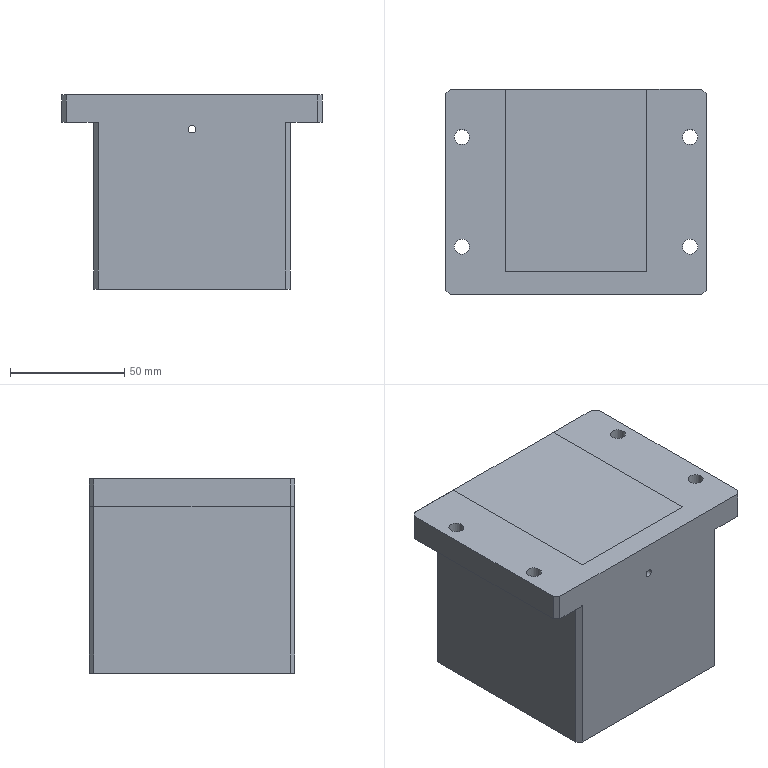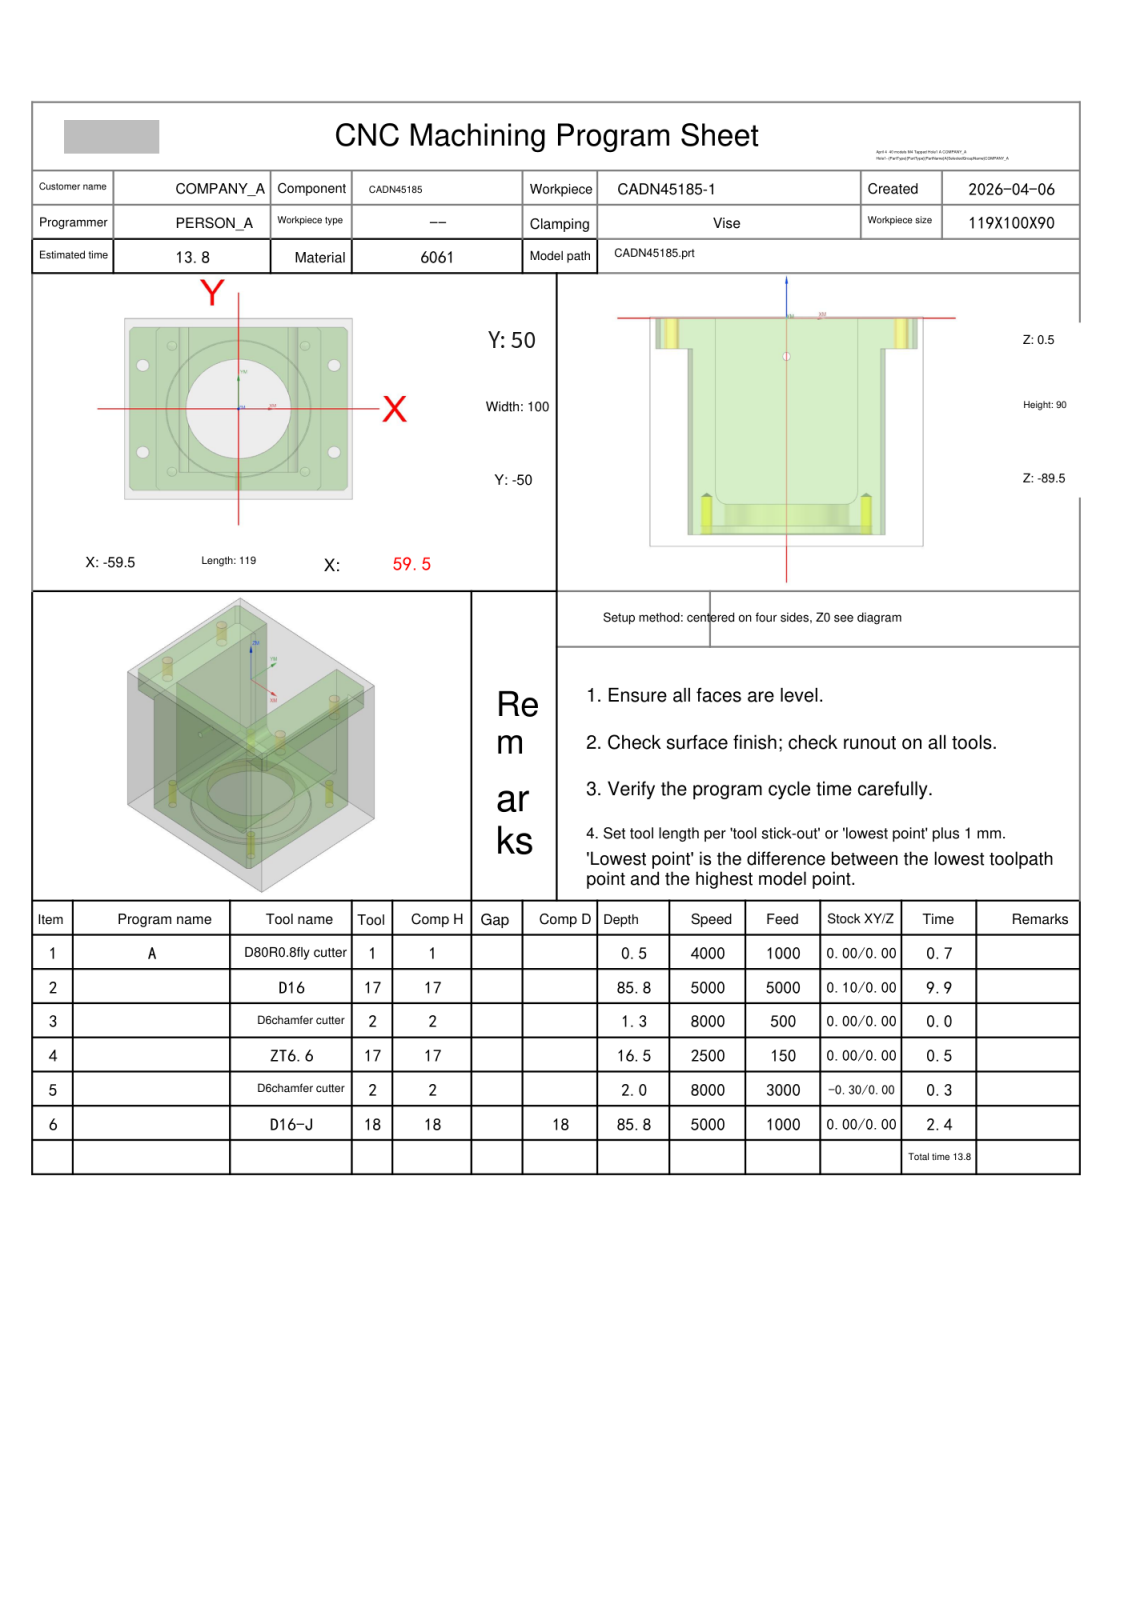NC program | NX | posted by the shop | part box 114 x 90 x 85 mm
Lines 35 to 791 of 2085:
N2 T17 M06
(D16  D=16. R=0. H=17 ce=0.10 di=0.00)
G00 G90 G54 X0.0 Y53.1 M03 S5000
G43 H17 Z20.
M08
Z.5
G01 X55. Z.404 F5000.
G02 X60.728 Y50.728 Z.393 I0.0 J-8.1
G01 X62.728 Y48.728 Z.388
G02 X65.1 Y43. Z.377 I-5.728 J-5.728
G01 Y-43. Z.226
G02 X62.728 Y-48.728 Z.215 I-8.1 J0.0
G01 X60.728 Y-50.728 Z.21
G02 X55. Y-53.1 Z.199 I-5.728 J5.728
G01 X-55. Z.007
G02 X-60.728 Y-50.728 Z-.005 I0.0 J8.1
G01 X-62.728 Y-48.728 Z-.009
G02 X-65.1 Y-43. Z-.021 I5.728 J5.728
G01 Y43. Z-.171
G02 X-62.728 Y48.728 Z-.182 I8.1 J0.0
G01 X-60.728 Y50.728 Z-.187
G02 X-55. Y53.1 Z-.198 I5.728 J-5.728
G01 X55. Z-.391
G02 X60.728 Y50.728 Z-.402 I0.0 J-8.1
G01 X62.728 Y48.728 Z-.407
G02 X65.1 Y43. Z-.418 I-5.728 J-5.728
G01 Y-43. Z-.568
G02 X62.728 Y-48.728 Z-.579 I-8.1 J0.0
G01 X60.728 Y-50.728 Z-.584
G02 X55. Y-53.1 Z-.595 I-5.728 J5.728
G01 X-55. Z-.788
G02 X-60.728 Y-50.728 Z-.799 I0.0 J8.1
G01 X-62.728 Y-48.728 Z-.804
G02 X-65.1 Y-43. Z-.815 I5.728 J5.728
G01 Y43. Z-.965
G02 X-62.728 Y48.728 Z-.977 I8.1 J0.0
G01 X-60.728 Y50.728 Z-.982
G02 X-55. Y53.1 Z-.993 I5.728 J-5.728
G01 X55. Z-1.185
G02 X60.728 Y50.728 Z-1.196 I0.0 J-8.1
G01 X62.728 Y48.728 Z-1.201
G02 X65.1 Y43. Z-1.212 I-5.728 J-5.728
G01 Y-43. Z-1.363
G02 X62.728 Y-48.728 Z-1.374 I-8.1 J0.0
G01 X60.728 Y-50.728 Z-1.379
G02 X55. Y-53.1 Z-1.39 I-5.728 J5.728
G01 X-55. Z-1.582
G02 X-60.728 Y-50.728 Z-1.593 I0.0 J8.1
G01 X-62.728 Y-48.728 Z-1.598
G02 X-65.1 Y-43. Z-1.61 I5.728 J5.728
G01 Y43. Z-1.76
G02 X-62.728 Y48.728 Z-1.771 I8.1 J0.0
G01 X-60.728 Y50.728 Z-1.776
G02 X-55. Y53.1 Z-1.787 I5.728 J-5.728
G01 X55. Z-1.98
G02 X60.728 Y50.728 Z-1.991 I0.0 J-8.1
G01 X62.728 Y48.728 Z-1.996
G02 X65.1 Y43. Z-2.007 I-5.728 J-5.728
G01 Y-43. Z-2.157
G02 X62.728 Y-48.728 Z-2.168 I-8.1 J0.0
G01 X60.728 Y-50.728 Z-2.173
G02 X55. Y-53.1 Z-2.184 I-5.728 J5.728
G01 X-55. Z-2.377
G02 X-60.728 Y-50.728 Z-2.388 I0.0 J8.1
G01 X-62.728 Y-48.728 Z-2.393
G02 X-65.1 Y-43. Z-2.404 I5.728 J5.728
G01 Y43. Z-2.554
G02 X-62.728 Y48.728 Z-2.566 I8.1 J0.0
G01 X-60.728 Y50.728 Z-2.57
G02 X-55. Y53.1 Z-2.582 I5.728 J-5.728
G01 X55. Z-2.774
G02 X60.728 Y50.728 Z-2.785 I0.0 J-8.1
G01 X62.728 Y48.728 Z-2.79
G02 X65.1 Y43. Z-2.801 I-5.728 J-5.728
G01 Y-43. Z-2.952
G02 X62.728 Y-48.728 Z-2.963 I-8.1 J0.0
G01 X60.728 Y-50.728 Z-2.968
G02 X55. Y-53.1 Z-2.979 I-5.728 J5.728
G01 X-55. Z-3.171
G02 X-60.728 Y-50.728 Z-3.182 I0.0 J8.1
G01 X-62.728 Y-48.728 Z-3.187
G02 X-65.1 Y-43. Z-3.198 I5.728 J5.728
G01 Y43. Z-3.349
G02 X-62.728 Y48.728 Z-3.36 I8.1 J0.0
G01 X-60.728 Y50.728 Z-3.365
G02 X-55. Y53.1 Z-3.376 I5.728 J-5.728
G01 X55. Z-3.568
G02 X60.728 Y50.728 Z-3.58 I0.0 J-8.1
G01 X62.728 Y48.728 Z-3.584
G02 X65.1 Y43. Z-3.596 I-5.728 J-5.728
G01 Y-43. Z-3.746
G02 X62.728 Y-48.728 Z-3.757 I-8.1 J0.0
G01 X60.728 Y-50.728 Z-3.762
G02 X55. Y-53.1 Z-3.773 I-5.728 J5.728
G01 X-55. Z-3.966
G02 X-60.728 Y-50.728 Z-3.977 I0.0 J8.1
G01 X-62.728 Y-48.728 Z-3.982
G02 X-65.1 Y-43. Z-3.993 I5.728 J5.728
G01 Y43. Z-4.143
G02 X-62.728 Y48.728 Z-4.154 I8.1 J0.0
G01 X-60.728 Y50.728 Z-4.159
G02 X-55. Y53.1 Z-4.17 I5.728 J-5.728
G01 X55. Z-4.363
G02 X60.728 Y50.728 Z-4.374 I0.0 J-8.1
G01 X62.728 Y48.728 Z-4.379
G02 X65.1 Y43. Z-4.39 I-5.728 J-5.728
G01 Y-43. Z-4.54
G02 X62.728 Y-48.728 Z-4.552 I-8.1 J0.0
G01 X60.728 Y-50.728 Z-4.557
G02 X55. Y-53.1 Z-4.568 I-5.728 J5.728
G01 X-55. Z-4.76
G02 X-60.728 Y-50.728 Z-4.771 I0.0 J8.1
G01 X-62.728 Y-48.728 Z-4.776
G02 X-65.1 Y-43. Z-4.787 I5.728 J5.728
G01 Y43. Z-4.938
G02 X-62.728 Y48.728 Z-4.949 I8.1 J0.0
G01 X-60.728 Y50.728 Z-4.954
G02 X-55. Y53.1 Z-4.965 I5.728 J-5.728
G01 X55. Z-5.157
G02 X60.728 Y50.728 Z-5.168 I0.0 J-8.1
G01 X62.728 Y48.728 Z-5.173
G02 X65.1 Y43. Z-5.185 I-5.728 J-5.728
G01 Y-43. Z-5.335
G02 X62.728 Y-48.728 Z-5.346 I-8.1 J0.0
G01 X60.728 Y-50.728 Z-5.351
G02 X55. Y-53.1 Z-5.362 I-5.728 J5.728
G01 X-55. Z-5.555
G02 X-60.728 Y-50.728 Z-5.566 I0.0 J8.1
G01 X-62.728 Y-48.728 Z-5.571
G02 X-65.1 Y-43. Z-5.582 I5.728 J5.728
G01 Y43. Z-5.732
G02 X-62.728 Y48.728 Z-5.743 I8.1 J0.0
G01 X-60.728 Y50.728 Z-5.748
G02 X-55. Y53.1 Z-5.759 I5.728 J-5.728
G01 X55. Z-5.952
G02 X60.728 Y50.728 Z-5.963 I0.0 J-8.1
G01 X62.728 Y48.728 Z-5.968
G02 X65.1 Y43. Z-5.979 I-5.728 J-5.728
G01 Y-43. Z-6.129
G02 X62.728 Y-48.728 Z-6.141 I-8.1 J0.0
G01 X60.728 Y-50.728 Z-6.145
G02 X55. Y-53.1 Z-6.157 I-5.728 J5.728
G01 X-55. Z-6.349
G02 X-60.728 Y-50.728 Z-6.36 I0.0 J8.1
G01 X-62.728 Y-48.728 Z-6.365
G02 X-65.1 Y-43. Z-6.376 I5.728 J5.728
G01 Y43. Z-6.527
G02 X-62.728 Y48.728 Z-6.538 I8.1 J0.0
G01 X-60.728 Y50.728 Z-6.543
G02 X-55. Y53.1 Z-6.554 I5.728 J-5.728
G01 X55. Z-6.746
G02 X60.728 Y50.728 Z-6.757 I0.0 J-8.1
G01 X62.728 Y48.728 Z-6.762
G02 X65.1 Y43. Z-6.773 I-5.728 J-5.728
G01 Y-43. Z-6.924
G02 X62.728 Y-48.728 Z-6.935 I-8.1 J0.0
G01 X60.728 Y-50.728 Z-6.94
G02 X55. Y-53.1 Z-6.951 I-5.728 J5.728
G01 X-55. Z-7.143
G02 X-60.728 Y-50.728 Z-7.155 I0.0 J8.1
G01 X-62.728 Y-48.728 Z-7.159
G02 X-65.1 Y-43. Z-7.171 I5.728 J5.728
G01 Y43. Z-7.321
G02 X-62.728 Y48.728 Z-7.332 I8.1 J0.0
G01 X-60.728 Y50.728 Z-7.337
G02 X-55. Y53.1 Z-7.348 I5.728 J-5.728
G01 X55. Z-7.541
G02 X60.728 Y50.728 Z-7.552 I0.0 J-8.1
G01 X62.728 Y48.728 Z-7.557
G02 X65.1 Y43. Z-7.568 I-5.728 J-5.728
G01 Y-43. Z-7.718
G02 X62.728 Y-48.728 Z-7.729 I-8.1 J0.0
G01 X60.728 Y-50.728 Z-7.734
G02 X55. Y-53.1 Z-7.745 I-5.728 J5.728
G01 X-55. Z-7.938
G02 X-60.728 Y-50.728 Z-7.949 I0.0 J8.1
G01 X-62.728 Y-48.728 Z-7.954
G02 X-65.1 Y-43. Z-7.965 I5.728 J5.728
G01 Y43. Z-8.115
G02 X-62.728 Y48.728 Z-8.127 I8.1 J0.0
G01 X-60.728 Y50.728 Z-8.132
G02 X-55. Y53.1 Z-8.143 I5.728 J-5.728
G01 X55. Z-8.335
G02 X60.728 Y50.728 Z-8.346 I0.0 J-8.1
G01 X62.728 Y48.728 Z-8.351
G02 X65.1 Y43. Z-8.362 I-5.728 J-5.728
G01 Y-43. Z-8.513
G02 X62.728 Y-48.728 Z-8.524 I-8.1 J0.0
G01 X60.728 Y-50.728 Z-8.529
G02 X55. Y-53.1 Z-8.54 I-5.728 J5.728
G01 X-55. Z-8.732
G02 X-60.728 Y-50.728 Z-8.743 I0.0 J8.1
G01 X-62.728 Y-48.728 Z-8.748
G02 X-65.1 Y-43. Z-8.76 I5.728 J5.728
G01 Y43. Z-8.91
G02 X-62.728 Y48.728 Z-8.921 I8.1 J0.0
G01 X-60.728 Y50.728 Z-8.926
G02 X-55. Y53.1 Z-8.937 I5.728 J-5.728
G01 X55. Z-9.13
G02 X60.728 Y50.728 Z-9.141 I0.0 J-8.1
G01 X62.728 Y48.728 Z-9.146
G02 X65.1 Y43. Z-9.157 I-5.728 J-5.728
G01 Y-43. Z-9.307
G02 X62.728 Y-48.728 Z-9.318 I-8.1 J0.0
G01 X60.728 Y-50.728 Z-9.323
G02 X55. Y-53.1 Z-9.334 I-5.728 J5.728
G01 X-55. Z-9.527
G02 X-60.728 Y-50.728 Z-9.538 I0.0 J8.1
G01 X-62.728 Y-48.728 Z-9.543
G02 X-65.1 Y-43. Z-9.554 I5.728 J5.728
G01 Y43. Z-9.704
G02 X-62.728 Y48.728 Z-9.716 I8.1 J0.0
G01 X-60.728 Y50.728 Z-9.72
G02 X-55. Y53.1 Z-9.732 I5.728 J-5.728
G01 X55. Z-9.924
G02 X60.728 Y50.728 Z-9.935 I0.0 J-8.1
G01 X62.728 Y48.728 Z-9.94
G02 X65.1 Y43. Z-9.951 I-5.728 J-5.728
G01 Y-43. Z-10.102
G02 X62.728 Y-48.728 Z-10.113 I-8.1 J0.0
G01 X60.728 Y-50.728 Z-10.118
G02 X55. Y-53.1 Z-10.129 I-5.728 J5.728
G01 X-55. Z-10.321
G02 X-60.728 Y-50.728 Z-10.332 I0.0 J8.1
G01 X-62.728 Y-48.728 Z-10.337
G02 X-65.1 Y-43. Z-10.348 I5.728 J5.728
G01 Y43. Z-10.499
G02 X-62.728 Y48.728 Z-10.51 I8.1 J0.0
G01 X-60.728 Y50.728 Z-10.515
G02 X-55. Y53.1 Z-10.526 I5.728 J-5.728
G01 X55. Z-10.718
G02 X60.728 Y50.728 Z-10.73 I0.0 J-8.1
G01 X62.728 Y48.728 Z-10.734
G02 X65.1 Y43. Z-10.746 I-5.728 J-5.728
G01 Y-43. Z-10.896
G02 X62.728 Y-48.728 Z-10.907 I-8.1 J0.0
G01 X60.728 Y-50.728 Z-10.912
G02 X55. Y-53.1 Z-10.923 I-5.728 J5.728
G01 X-55. Z-11.116
G02 X-60.728 Y-50.728 Z-11.127 I0.0 J8.1
G01 X-62.728 Y-48.728 Z-11.132
G02 X-65.1 Y-43. Z-11.143 I5.728 J5.728
G01 Y43. Z-11.293
G02 X-62.728 Y48.728 Z-11.304 I8.1 J0.0
G01 X-60.728 Y50.728 Z-11.309
G02 X-55. Y53.1 Z-11.32 I5.728 J-5.728
G01 X55. Z-11.513
G02 X60.728 Y50.728 Z-11.524 I0.0 J-8.1
G01 X62.728 Y48.728 Z-11.529
G02 X65.1 Y43. Z-11.54 I-5.728 J-5.728
G01 Y-43. Z-11.69
G02 X62.728 Y-48.728 Z-11.702 I-8.1 J0.0
G01 X60.728 Y-50.728 Z-11.707
G02 X55. Y-53.1 Z-11.718 I-5.728 J5.728
G01 X-55. Z-11.91
G02 X-60.728 Y-50.728 Z-11.921 I0.0 J8.1
G01 X-62.728 Y-48.728 Z-11.926
G02 X-65.1 Y-43. Z-11.937 I5.728 J5.728
G01 Y43. Z-12.088
G02 X-62.728 Y48.728 Z-12.099 I8.1 J0.0
G01 X-60.728 Y50.728 Z-12.104
G02 X-55. Y53.1 Z-12.115 I5.728 J-5.728
G01 X55. Z-12.307
G02 X60.728 Y50.728 Z-12.318 I0.0 J-8.1
G01 X62.728 Y48.728 Z-12.323
G02 X65.1 Y43. Z-12.335 I-5.728 J-5.728
G01 Y-43. Z-12.485
G02 X62.728 Y-48.728 Z-12.496 I-8.1 J0.0
G01 X60.728 Y-50.728 Z-12.501
G02 X55. Y-53.1 Z-12.512 I-5.728 J5.728
G01 X-55. Z-12.705
G02 X-60.728 Y-50.728 Z-12.716 I0.0 J8.1
G01 X-62.728 Y-48.728 Z-12.721
G02 X-65.1 Y-43. Z-12.732 I5.728 J5.728
G01 Y43. Z-12.882
G02 X-62.728 Y48.728 Z-12.893 I8.1 J0.0
G01 X-60.728 Y50.728 Z-12.898
G02 X-55. Y53.1 Z-12.909 I5.728 J-5.728
G01 X55. Z-13.102
G02 X60.728 Y50.728 Z-13.113 I0.0 J-8.1
G01 X62.728 Y48.728 Z-13.118
G02 X65.1 Y43. Z-13.129 I-5.728 J-5.728
G01 Y-43. Z-13.279
G02 X62.728 Y-48.728 Z-13.291 I-8.1 J0.0
G01 X60.728 Y-50.728 Z-13.295
G02 X55. Y-53.1 Z-13.307 I-5.728 J5.728
G01 X-55. Z-13.499
G02 X-60.728 Y-50.728 Z-13.51 I0.0 J8.1
G01 X-62.728 Y-48.728 Z-13.515
G02 X-65.1 Y-43. Z-13.526 I5.728 J5.728
G01 Y43. Z-13.677
G02 X-62.728 Y48.728 Z-13.688 I8.1 J0.0
G01 X-60.728 Y50.728 Z-13.693
G02 X-55. Y53.1 Z-13.704 I5.728 J-5.728
G01 X55. Z-13.896
G02 X60.728 Y50.728 Z-13.907 I0.0 J-8.1
G01 X62.728 Y48.728 Z-13.912
G02 X65.1 Y43. Z-13.923 I-5.728 J-5.728
G01 Y-43. Z-14.074
G02 X62.728 Y-48.728 Z-14.085 I-8.1 J0.0
G01 X60.728 Y-50.728 Z-14.09
G02 X55. Y-53.1 Z-14.101 I-5.728 J5.728
G01 X-55. Z-14.293
G02 X-60.728 Y-50.728 Z-14.305 I0.0 J8.1
G01 X-62.728 Y-48.728 Z-14.309
G02 X-65.1 Y-43. Z-14.321 I5.728 J5.728
G01 Y43. Z-14.471
G02 X-62.728 Y48.728 Z-14.482 I8.1 J0.0
G01 X-60.728 Y50.728 Z-14.487
G02 X-55. Y53.1 Z-14.498 I5.728 J-5.728
G01 X55. Z-14.691
G02 X60.728 Y50.728 Z-14.702 I0.0 J-8.1
G01 X62.728 Y48.728 Z-14.707
G02 X65.1 Y43. Z-14.718 I-5.728 J-5.728
G01 Y-43. Z-14.868
G02 X62.728 Y-48.728 Z-14.879 I-8.1 J0.0
G01 X60.728 Y-50.728 Z-14.884
G02 X55. Y-53.1 Z-14.895 I-5.728 J5.728
G01 X-55. Z-15.088
G02 X-60.728 Y-50.728 Z-15.099 I0.0 J8.1
G01 X-62.728 Y-48.728 Z-15.104
G02 X-65.1 Y-43. Z-15.115 I5.728 J5.728
G01 Y43. Z-15.265
G02 X-62.728 Y48.728 Z-15.277 I8.1 J0.0
G01 X-60.728 Y50.728 Z-15.282
G02 X-55. Y53.1 Z-15.293 I5.728 J-5.728
G01 X55. Z-15.485
G02 X60.728 Y50.728 Z-15.496 I0.0 J-8.1
G01 X62.728 Y48.728 Z-15.501
G02 X65.1 Y43. Z-15.512 I-5.728 J-5.728
G01 Y-43. Z-15.663
G02 X62.728 Y-48.728 Z-15.674 I-8.1 J0.0
G01 X60.728 Y-50.728 Z-15.679
G02 X55. Y-53.1 Z-15.69 I-5.728 J5.728
G01 X-55. Z-15.882
G02 X-60.728 Y-50.728 Z-15.893 I0.0 J8.1
G01 X-62.728 Y-48.728 Z-15.898
G02 X-65.1 Y-43. Z-15.91 I5.728 J5.728
G01 Y43. Z-16.06
G02 X-62.728 Y48.728 Z-16.071 I8.1 J0.0
G01 X-60.728 Y50.728 Z-16.076
G02 X-55. Y53.1 Z-16.087 I5.728 J-5.728
G01 X55. Z-16.28
G02 X60.728 Y50.728 Z-16.291 I0.0 J-8.1
G01 X62.728 Y48.728 Z-16.296
G02 X65.1 Y43. Z-16.307 I-5.728 J-5.728
G01 Y-43. Z-16.457
G02 X62.728 Y-48.728 Z-16.468 I-8.1 J0.0
G01 X60.728 Y-50.728 Z-16.473
G02 X55. Y-53.1 Z-16.484 I-5.728 J5.728
G01 X-55. Z-16.677
G02 X-60.728 Y-50.728 Z-16.688 I0.0 J8.1
G01 X-62.728 Y-48.728 Z-16.693
G02 X-65.1 Y-43. Z-16.704 I5.728 J5.728
G01 Y43. Z-16.854
G02 X-62.728 Y48.728 Z-16.866 I8.1 J0.0
G01 X-60.728 Y50.728 Z-16.87
G02 X-55. Y53.1 Z-16.882 I5.728 J-5.728
G01 X55. Z-17.074
G02 X60.728 Y50.728 Z-17.085 I0.0 J-8.1
G01 X62.728 Y48.728 Z-17.09
G02 X65.1 Y43. Z-17.101 I-5.728 J-5.728
G01 Y-43. Z-17.252
G02 X62.728 Y-48.728 Z-17.263 I-8.1 J0.0
G01 X60.728 Y-50.728 Z-17.268
G02 X55. Y-53.1 Z-17.279 I-5.728 J5.728
G01 X-55. Z-17.471
G02 X-60.728 Y-50.728 Z-17.482 I0.0 J8.1
G01 X-62.728 Y-48.728 Z-17.487
G02 X-65.1 Y-43. Z-17.498 I5.728 J5.728
G01 Y43. Z-17.649
G02 X-62.728 Y48.728 Z-17.66 I8.1 J0.0
G01 X-60.728 Y50.728 Z-17.665
G02 X-55. Y53.1 Z-17.676 I5.728 J-5.728
G01 X55. Z-17.868
G02 X60.728 Y50.728 Z-17.88 I0.0 J-8.1
G01 X62.728 Y48.728 Z-17.884
G02 X65.1 Y43. Z-17.896 I-5.728 J-5.728
G01 Y-43. Z-18.046
G02 X62.728 Y-48.728 Z-18.057 I-8.1 J0.0
G01 X60.728 Y-50.728 Z-18.062
G02 X55. Y-53.1 Z-18.073 I-5.728 J5.728
G01 X-55. Z-18.266
G02 X-60.728 Y-50.728 Z-18.277 I0.0 J8.1
G01 X-62.728 Y-48.728 Z-18.282
G02 X-65.1 Y-43. Z-18.293 I5.728 J5.728
G01 Y43. Z-18.443
G02 X-62.728 Y48.728 Z-18.454 I8.1 J0.0
G01 X-60.728 Y50.728 Z-18.459
G02 X-55. Y53.1 Z-18.47 I5.728 J-5.728
G01 X55. Z-18.663
G02 X60.728 Y50.728 Z-18.674 I0.0 J-8.1
G01 X62.728 Y48.728 Z-18.679
G02 X65.1 Y43. Z-18.69 I-5.728 J-5.728
G01 Y-43. Z-18.84
G02 X62.728 Y-48.728 Z-18.852 I-8.1 J0.0
G01 X60.728 Y-50.728 Z-18.857
G02 X55. Y-53.1 Z-18.868 I-5.728 J5.728
G01 X-55. Z-19.06
G02 X-60.728 Y-50.728 Z-19.071 I0.0 J8.1
G01 X-62.728 Y-48.728 Z-19.076
G02 X-65.1 Y-43. Z-19.087 I5.728 J5.728
G01 Y43. Z-19.238
G02 X-62.728 Y48.728 Z-19.249 I8.1 J0.0
G01 X-60.728 Y50.728 Z-19.254
G02 X-55. Y53.1 Z-19.265 I5.728 J-5.728
G01 X55. Z-19.457
G02 X60.728 Y50.728 Z-19.468 I0.0 J-8.1
G01 X62.728 Y48.728 Z-19.473
G02 X65.1 Y43. Z-19.485 I-5.728 J-5.728
G01 Y-43. Z-19.635
G02 X62.728 Y-48.728 Z-19.646 I-8.1 J0.0
G01 X60.728 Y-50.728 Z-19.651
G02 X55. Y-53.1 Z-19.662 I-5.728 J5.728
G01 X-55. Z-19.855
G02 X-60.728 Y-50.728 Z-19.866 I0.0 J8.1
G01 X-62.728 Y-48.728 Z-19.871
G02 X-65.1 Y-43. Z-19.882 I5.728 J5.728
G01 Y43. Z-20.032
G02 X-62.728 Y48.728 Z-20.043 I8.1 J0.0
G01 X-60.728 Y50.728 Z-20.048
G02 X-55. Y53.1 Z-20.059 I5.728 J-5.728
G01 X55. Z-20.252
G02 X60.728 Y50.728 Z-20.263 I0.0 J-8.1
G01 X62.728 Y48.728 Z-20.268
G02 X65.1 Y43. Z-20.279 I-5.728 J-5.728
G01 Y-43. Z-20.429
G02 X62.728 Y-48.728 Z-20.441 I-8.1 J0.0
G01 X60.728 Y-50.728 Z-20.445
G02 X55. Y-53.1 Z-20.457 I-5.728 J5.728
G01 X-55. Z-20.649
G02 X-60.728 Y-50.728 Z-20.66 I0.0 J8.1
G01 X-62.728 Y-48.728 Z-20.665
G02 X-65.1 Y-43. Z-20.676 I5.728 J5.728
G01 Y43. Z-20.827
G02 X-62.728 Y48.728 Z-20.838 I8.1 J0.0
G01 X-60.728 Y50.728 Z-20.843
G02 X-55. Y53.1 Z-20.854 I5.728 J-5.728
G01 X55. Z-21.046
G02 X60.728 Y50.728 Z-21.057 I0.0 J-8.1
G01 X62.728 Y48.728 Z-21.062
G02 X65.1 Y43. Z-21.073 I-5.728 J-5.728
G01 Y-43. Z-21.224
G02 X62.728 Y-48.728 Z-21.235 I-8.1 J0.0
G01 X60.728 Y-50.728 Z-21.24
G02 X55. Y-53.1 Z-21.251 I-5.728 J5.728
G01 X-55. Z-21.443
G02 X-60.728 Y-50.728 Z-21.455 I0.0 J8.1
G01 X-62.728 Y-48.728 Z-21.459
G02 X-65.1 Y-43. Z-21.471 I5.728 J5.728
G01 Y43. Z-21.621
G02 X-62.728 Y48.728 Z-21.632 I8.1 J0.0
G01 X-60.728 Y50.728 Z-21.637
G02 X-55. Y53.1 Z-21.648 I5.728 J-5.728
G01 X55. Z-21.841
G02 X60.728 Y50.728 Z-21.852 I0.0 J-8.1
G01 X62.728 Y48.728 Z-21.857
G02 X65.1 Y43. Z-21.868 I-5.728 J-5.728
G01 Y-43. Z-22.018
G02 X62.728 Y-48.728 Z-22.029 I-8.1 J0.0
G01 X60.728 Y-50.728 Z-22.034
G02 X55. Y-53.1 Z-22.045 I-5.728 J5.728
G01 X-55. Z-22.238
G02 X-60.728 Y-50.728 Z-22.249 I0.0 J8.1
G01 X-62.728 Y-48.728 Z-22.254
G02 X-65.1 Y-43. Z-22.265 I5.728 J5.728
G01 Y43. Z-22.415
G02 X-62.728 Y48.728 Z-22.427 I8.1 J0.0
G01 X-60.728 Y50.728 Z-22.432
G02 X-55. Y53.1 Z-22.443 I5.728 J-5.728
G01 X55. Z-22.635
G02 X60.728 Y50.728 Z-22.646 I0.0 J-8.1
G01 X62.728 Y48.728 Z-22.651
G02 X65.1 Y43. Z-22.662 I-5.728 J-5.728
G01 Y-43. Z-22.813
G02 X62.728 Y-48.728 Z-22.824 I-8.1 J0.0
G01 X60.728 Y-50.728 Z-22.829
G02 X55. Y-53.1 Z-22.84 I-5.728 J5.728
G01 X-55. Z-23.032
G02 X-60.728 Y-50.728 Z-23.043 I0.0 J8.1
G01 X-62.728 Y-48.728 Z-23.048
G02 X-65.1 Y-43. Z-23.06 I5.728 J5.728
G01 Y43. Z-23.21
G02 X-62.728 Y48.728 Z-23.221 I8.1 J0.0
G01 X-60.728 Y50.728 Z-23.226
G02 X-55. Y53.1 Z-23.237 I5.728 J-5.728
G01 X55. Z-23.43
G02 X60.728 Y50.728 Z-23.441 I0.0 J-8.1
G01 X62.728 Y48.728 Z-23.446
G02 X65.1 Y43. Z-23.457 I-5.728 J-5.728
G01 Y-43. Z-23.607
G02 X62.728 Y-48.728 Z-23.618 I-8.1 J0.0
G01 X60.728 Y-50.728 Z-23.623
G02 X55. Y-53.1 Z-23.634 I-5.728 J5.728
G01 X-55. Z-23.827
G02 X-60.728 Y-50.728 Z-23.838 I0.0 J8.1
G01 X-62.728 Y-48.728 Z-23.843
G02 X-65.1 Y-43. Z-23.854 I5.728 J5.728
G01 Y43. Z-24.004
G02 X-62.728 Y48.728 Z-24.016 I8.1 J0.0
G01 X-60.728 Y50.728 Z-24.02
G02 X-55. Y53.1 Z-24.032 I5.728 J-5.728
G01 X55. Z-24.224
G02 X60.728 Y50.728 Z-24.235 I0.0 J-8.1
G01 X62.728 Y48.728 Z-24.24
G02 X65.1 Y43. Z-24.251 I-5.728 J-5.728
G01 Y-43. Z-24.402
G02 X62.728 Y-48.728 Z-24.413 I-8.1 J0.0
G01 X60.728 Y-50.728 Z-24.418
G02 X55. Y-53.1 Z-24.429 I-5.728 J5.728
G01 X-55. Z-24.621
G02 X-60.728 Y-50.728 Z-24.632 I0.0 J8.1
G01 X-62.728 Y-48.728 Z-24.637
G02 X-65.1 Y-43. Z-24.648 I5.728 J5.728
G01 Y43. Z-24.799
G02 X-62.728 Y48.728 Z-24.81 I8.1 J0.0
G01 X-60.728 Y50.728 Z-24.815
G02 X-55. Y53.1 Z-24.826 I5.728 J-5.728
G01 X55. Z-25.018
G02 X60.728 Y50.728 Z-25.03 I0.0 J-8.1
G01 X62.728 Y48.728 Z-25.034
G02 X65.1 Y43. Z-25.046 I-5.728 J-5.728
G01 Y-43. Z-25.196
G02 X62.728 Y-48.728 Z-25.207 I-8.1 J0.0
G01 X60.728 Y-50.728 Z-25.212
G02 X55. Y-53.1 Z-25.223 I-5.728 J5.728
G01 X-55. Z-25.416
G02 X-60.728 Y-50.728 Z-25.427 I0.0 J8.1
G01 X-62.728 Y-48.728 Z-25.432
G02 X-65.1 Y-43. Z-25.443 I5.728 J5.728
G01 Y43. Z-25.593
G02 X-62.728 Y48.728 Z-25.604 I8.1 J0.0
G01 X-60.728 Y50.728 Z-25.609
G02 X-55. Y53.1 Z-25.62 I5.728 J-5.728
G01 X55. Z-25.813
G02 X60.728 Y50.728 Z-25.824 I0.0 J-8.1
G01 X62.728 Y48.728 Z-25.829
G02 X65.1 Y43. Z-25.84 I-5.728 J-5.728
G01 Y-43. Z-25.99
G02 X62.728 Y-48.728 Z-26.002 I-8.1 J0.0
G01 X60.728 Y-50.728 Z-26.007
G02 X55. Y-53.1 Z-26.018 I-5.728 J5.728
G01 X-55. Z-26.21
G02 X-60.728 Y-50.728 Z-26.221 I0.0 J8.1
G01 X-62.728 Y-48.728 Z-26.226
G02 X-65.1 Y-43. Z-26.237 I5.728 J5.728
G01 Y43. Z-26.388
G02 X-62.728 Y48.728 Z-26.399 I8.1 J0.0
G01 X-60.728 Y50.728 Z-26.404
G02 X-55. Y53.1 Z-26.415 I5.728 J-5.728
G01 X55. Z-26.607
G02 X60.728 Y50.728 Z-26.618 I0.0 J-8.1
G01 X62.728 Y48.728 Z-26.623
G02 X65.1 Y43. Z-26.635 I-5.728 J-5.728
G01 Y-43. Z-26.785
G02 X62.728 Y-48.728 Z-26.796 I-8.1 J0.0
G01 X60.728 Y-50.728 Z-26.801
G02 X55. Y-53.1 Z-26.812 I-5.728 J5.728
G01 X-55. Z-27.005
G02 X-60.728 Y-50.728 Z-27.016 I0.0 J8.1
G01 X-62.728 Y-48.728 Z-27.021
G02 X-65.1 Y-43. Z-27.032 I5.728 J5.728
G01 Y43. Z-27.182
G02 X-62.728 Y48.728 Z-27.193 I8.1 J0.0
G01 X-60.728 Y50.728 Z-27.198
G02 X-55. Y53.1 Z-27.209 I5.728 J-5.728
G01 X55. Z-27.402
G02 X60.728 Y50.728 Z-27.413 I0.0 J-8.1
G01 X62.728 Y48.728 Z-27.418
G02 X65.1 Y43. Z-27.429 I-5.728 J-5.728
G01 Y-43. Z-27.579
G02 X62.728 Y-48.728 Z-27.591 I-8.1 J0.0
G01 X60.728 Y-50.728 Z-27.595
G02 X55. Y-53.1 Z-27.607 I-5.728 J5.728
G01 X-55. Z-27.799
G02 X-60.728 Y-50.728 Z-27.81 I0.0 J8.1
G01 X-62.728 Y-48.728 Z-27.815
G02 X-65.1 Y-43. Z-27.826 I5.728 J5.728
G01 Y43. Z-27.977
G02 X-62.728 Y48.728 Z-27.988 I8.1 J0.0
G01 X-60.728 Y50.728 Z-27.993
G02 X-55. Y53.1 Z-28.004 I5.728 J-5.728
G01 X55. Z-28.196
G02 X60.728 Y50.728 Z-28.207 I0.0 J-8.1
G01 X62.728 Y48.728 Z-28.212
G02 X65.1 Y43. Z-28.223 I-5.728 J-5.728
G01 Y-43. Z-28.374
G02 X62.728 Y-48.728 Z-28.385 I-8.1 J0.0
G01 X60.728 Y-50.728 Z-28.39
G02 X55. Y-53.1 Z-28.401 I-5.728 J5.728
G01 X-55. Z-28.593
G02 X-60.728 Y-50.728 Z-28.605 I0.0 J8.1
G01 X-62.728 Y-48.728 Z-28.609
G02 X-65.1 Y-43. Z-28.621 I5.728 J5.728
G01 Y43. Z-28.771
G02 X-62.728 Y48.728 Z-28.782 I8.1 J0.0
G01 X-60.728 Y50.728 Z-28.787
G02 X-55. Y53.1 Z-28.798 I5.728 J-5.728
G01 X55. Z-28.991
G02 X60.728 Y50.728 Z-29.002 I0.0 J-8.1
G01 X62.728 Y48.728 Z-29.007
G02 X65.1 Y43. Z-29.018 I-5.728 J-5.728
G01 Y-43. Z-29.168
G02 X62.728 Y-48.728 Z-29.179 I-8.1 J0.0
G01 X60.728 Y-50.728 Z-29.184
G02 X55. Y-53.1 Z-29.195 I-5.728 J5.728
G01 X-55. Z-29.388
G02 X-60.728 Y-50.728 Z-29.399 I0.0 J8.1
G01 X-62.728 Y-48.728 Z-29.404
G02 X-65.1 Y-43. Z-29.415 I5.728 J5.728
G01 Y43. Z-29.565
G02 X-62.728 Y48.728 Z-29.577 I8.1 J0.0
G01 X-60.728 Y50.728 Z-29.582
G02 X-55. Y53.1 Z-29.593 I5.728 J-5.728
G01 X55. Z-29.785
G02 X60.728 Y50.728 Z-29.796 I0.0 J-8.1
G01 X62.728 Y48.728 Z-29.801
G02 X65.1 Y43. Z-29.812 I-5.728 J-5.728
G01 Y-43. Z-29.963
G02 X62.728 Y-48.728 Z-29.974 I-8.1 J0.0
G01 X60.728 Y-50.728 Z-29.979
G02 X55. Y-53.1 Z-29.99 I-5.728 J5.728
G01 X-55. Z-30.182
G02 X-60.728 Y-50.728 Z-30.193 I0.0 J8.1
G01 X-62.728 Y-48.728 Z-30.198
G02 X-65.1 Y-43. Z-30.21 I5.728 J5.728
G01 Y43. Z-30.36
G02 X-62.728 Y48.728 Z-30.371 I8.1 J0.0
G01 X-60.728 Y50.728 Z-30.376
G02 X-55. Y53.1 Z-30.387 I5.728 J-5.728
G01 X55. Z-30.58
G02 X60.728 Y50.728 Z-30.591 I0.0 J-8.1
G01 X62.728 Y48.728 Z-30.596
G02 X65.1 Y43. Z-30.607 I-5.728 J-5.728
G01 Y-43. Z-30.757
G02 X62.728 Y-48.728 Z-30.768 I-8.1 J0.0
G01 X60.728 Y-50.728 Z-30.773
G02 X55. Y-53.1 Z-30.784 I-5.728 J5.728
G01 X-55. Z-30.977
G02 X-60.728 Y-50.728 Z-30.988 I0.0 J8.1
G01 X-62.728 Y-48.728 Z-30.993
G02 X-65.1 Y-43. Z-31.004 I5.728 J5.728
G01 Y43. Z-31.154
G02 X-62.728 Y48.728 Z-31.166 I8.1 J0.0
G01 X-60.728 Y50.728 Z-31.17
G02 X-55. Y53.1 Z-31.182 I5.728 J-5.728
G01 X55. Z-31.374
G02 X60.728 Y50.728 Z-31.385 I0.0 J-8.1
G01 X62.728 Y48.728 Z-31.39
G02 X65.1 Y43. Z-31.401 I-5.728 J-5.728
G01 Y-43. Z-31.552
G02 X62.728 Y-48.728 Z-31.563 I-8.1 J0.0
G01 X60.728 Y-50.728 Z-31.568
G02 X55. Y-53.1 Z-31.579 I-5.728 J5.728
G01 X-55. Z-31.771
G02 X-60.728 Y-50.728 Z-31.782 I0.0 J8.1
G01 X-62.728 Y-48.728 Z-31.787
G02 X-65.1 Y-43. Z-31.798 I5.728 J5.728
G01 Y43. Z-31.949
G02 X-62.728 Y48.728 Z-31.96 I8.1 J0.0
G01 X-60.728 Y50.728 Z-31.965
G02 X-55. Y53.1 Z-31.976 I5.728 J-5.728
G01 X55. Z-32.168
G02 X60.728 Y50.728 Z-32.18 I0.0 J-8.1
G01 X62.728 Y48.728 Z-32.184
G02 X65.1 Y43. Z-32.196 I-5.728 J-5.728
G01 Y-43. Z-32.346
G02 X62.728 Y-48.728 Z-32.357 I-8.1 J0.0
G01 X60.728 Y-50.728 Z-32.362
G02 X55. Y-53.1 Z-32.373 I-5.728 J5.728
G01 X-55. Z-32.566
G02 X-60.728 Y-50.728 Z-32.577 I0.0 J8.1
G01 X-62.728 Y-48.728 Z-32.582
G02 X-65.1 Y-43. Z-32.593 I5.728 J5.728
G01 Y43. Z-32.743
G02 X-62.728 Y48.728 Z-32.754 I8.1 J0.0
G01 X-60.728 Y50.728 Z-32.759
G02 X-55. Y53.1 Z-32.77 I5.728 J-5.728
G01 X55. Z-32.963
G02 X60.728 Y50.728 Z-32.974 I0.0 J-8.1
G01 X62.728 Y48.728 Z-32.979
G02 X65.1 Y43. Z-32.99 I-5.728 J-5.728
G01 Y-43. Z-33.14
G02 X62.728 Y-48.728 Z-33.152 I-8.1 J0.0
G01 X60.728 Y-50.728 Z-33.157
G02 X55. Y-53.1 Z-33.168 I-5.728 J5.728
G01 X-55. Z-33.36
G02 X-60.728 Y-50.728 Z-33.371 I0.0 J8.1
G01 X-62.728 Y-48.728 Z-33.376
G02 X-65.1 Y-43. Z-33.387 I5.728 J5.728
G01 Y43. Z-33.538
G02 X-62.728 Y48.728 Z-33.549 I8.1 J0.0
G01 X-60.728 Y50.728 Z-33.554
G02 X-55. Y53.1 Z-33.565 I5.728 J-5.728
G01 X55. Z-33.757
G02 X60.728 Y50.728 Z-33.768 I0.0 J-8.1
G01 X62.728 Y48.728 Z-33.773
G02 X65.1 Y43. Z-33.785 I-5.728 J-5.728
G01 Y-43. Z-33.935
G02 X62.728 Y-48.728 Z-33.946 I-8.1 J0.0
G01 X60.728 Y-50.728 Z-33.951
G02 X55. Y-53.1 Z-33.962 I-5.728 J5.728
G01 X-55. Z-34.155
G02 X-60.728 Y-50.728 Z-34.166 I0.0 J8.1
G01 X-62.728 Y-48.728 Z-34.171
G02 X-65.1 Y-43. Z-34.182 I5.728 J5.728
G01 Y43. Z-34.332
G02 X-62.728 Y48.728 Z-34.343 I8.1 J0.0
G01 X-60.728 Y50.728 Z-34.348
G02 X-55. Y53.1 Z-34.359 I5.728 J-5.728
G01 X55. Z-34.552
G02 X60.728 Y50.728 Z-34.563 I0.0 J-8.1
G01 X62.728 Y48.728 Z-34.568
G02 X65.1 Y43. Z-34.579 I-5.728 J-5.728
G01 Y-43. Z-34.729
G02 X62.728 Y-48.728 Z-34.741 I-8.1 J0.0
G01 X60.728 Y-50.728 Z-34.745
G02 X55. Y-53.1 Z-34.757 I-5.728 J5.728
G01 X-55. Z-34.949
G02 X-60.728 Y-50.728 Z-34.96 I0.0 J8.1
G01 X-62.728 Y-48.728 Z-34.965
G02 X-65.1 Y-43. Z-34.976 I5.728 J5.728
G01 Y43. Z-35.127
G02 X-62.728 Y48.728 Z-35.138 I8.1 J0.0
G01 X-60.728 Y50.728 Z-35.143
G02 X-55. Y53.1 Z-35.154 I5.728 J-5.728
G01 X55. Z-35.346
G02 X60.728 Y50.728 Z-35.357 I0.0 J-8.1
G01 X62.728 Y48.728 Z-35.362
G02 X65.1 Y43. Z-35.373 I-5.728 J-5.728
G01 Y-43. Z-35.524
G02 X62.728 Y-48.728 Z-35.535 I-8.1 J0.0
G01 X60.728 Y-50.728 Z-35.54
G02 X55. Y-53.1 Z-35.551 I-5.728 J5.728
G01 X-55. Z-35.743
G02 X-60.728 Y-50.728 Z-35.755 I0.0 J8.1
G01 X-62.728 Y-48.728 Z-35.759
G02 X-65.1 Y-43. Z-35.771 I5.728 J5.728
G01 Y43. Z-35.921
G02 X-62.728 Y48.728 Z-35.932 I8.1 J0.0
G01 X-60.728 Y50.728 Z-35.937
G02 X-55. Y53.1 Z-35.948 I5.728 J-5.728
G01 X55. Z-36.141
G02 X60.728 Y50.728 Z-36.152 I0.0 J-8.1
G01 X62.728 Y48.728 Z-36.157
G02 X65.1 Y43. Z-36.168 I-5.728 J-5.728
G01 Y-43. Z-36.318
G02 X62.728 Y-48.728 Z-36.329 I-8.1 J0.0
G01 X60.728 Y-50.728 Z-36.334
G02 X55. Y-53.1 Z-36.345 I-5.728 J5.728
G01 X-55. Z-36.538
G02 X-60.728 Y-50.728 Z-36.549 I0.0 J8.1
G01 X-62.728 Y-48.728 Z-36.554
G02 X-65.1 Y-43. Z-36.565 I5.728 J5.728
G01 Y43. Z-36.715
G02 X-62.728 Y48.728 Z-36.727 I8.1 J0.0
G01 X-60.728 Y50.728 Z-36.732